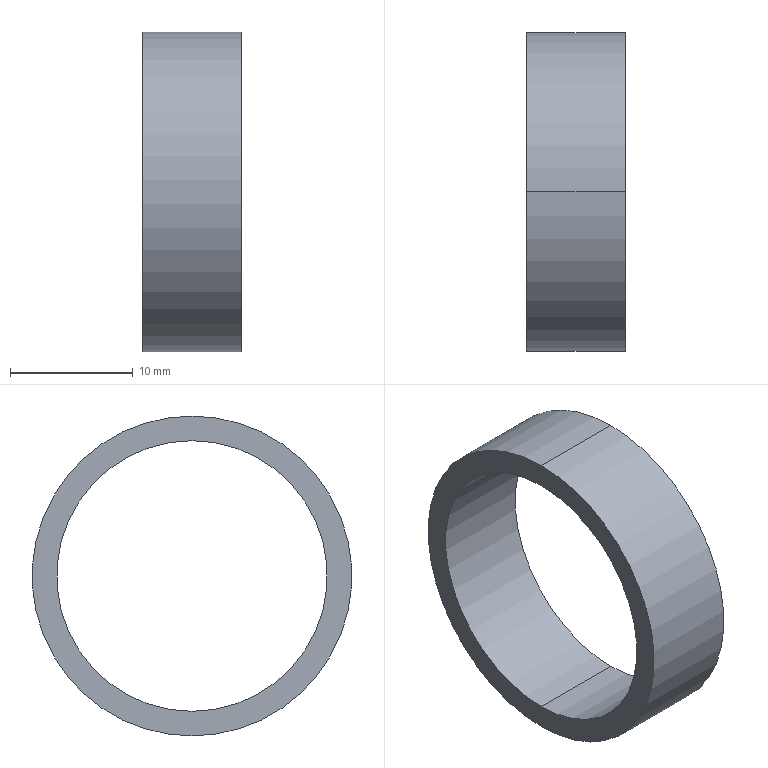Part | SolidWorks | features BaseBody 1 | 1 solid | 6 faces | box 8 x 26 x 26 mm | volume 1206 mm3 | cylinder 4 | plane 2 | commonest cylinder face diameters 22 x2 26 x2
STEP:
#1=CARTESIAN_POINT('',(-4.,0.,-13.));
#2=VERTEX_POINT('',#1);
#3=CARTESIAN_POINT('',(-4.,0.,13.));
#4=VERTEX_POINT('',#3);
#5=CARTESIAN_POINT('',(-4.,0.,0.));
#6=DIRECTION('',(1.,0.,0.));
#7=DIRECTION('',(0.,0.,-1.));
#8=AXIS2_PLACEMENT_3D('',#5,#6,#7);
#9=CIRCLE('',#8,13.);
#10=EDGE_CURVE('',#2,#4,#9,.T.);
#11=ORIENTED_EDGE('',*,*,#10,.T.);
#12=CARTESIAN_POINT('',(4.,0.,13.));
#13=VERTEX_POINT('',#12);
#14=CARTESIAN_POINT('',(-4.,0.,13.));
#15=DIRECTION('',(1.,0.,0.));
#16=VECTOR('',#15,1000.);
#17=LINE('',#14,#16);
#18=EDGE_CURVE('',#4,#13,#17,.T.);
#19=ORIENTED_EDGE('',*,*,#18,.T.);
#20=CARTESIAN_POINT('',(4.,0.,-13.));
#21=VERTEX_POINT('',#20);
#22=CARTESIAN_POINT('',(4.,0.,0.));
#23=DIRECTION('',(-1.,0.,0.));
#24=DIRECTION('',(0.,0.,-1.));
#25=AXIS2_PLACEMENT_3D('',#22,#23,#24);
#26=CIRCLE('',#25,13.);
#27=EDGE_CURVE('',#13,#21,#26,.T.);
#28=ORIENTED_EDGE('',*,*,#27,.T.);
#29=CARTESIAN_POINT('',(-4.,0.,-13.));
#30=DIRECTION('',(1.,0.,0.));
#31=VECTOR('',#30,1000.);
#32=LINE('',#29,#31);
#33=EDGE_CURVE('',#2,#21,#32,.T.);
#34=ORIENTED_EDGE('',*,*,#33,.F.);
#35=EDGE_LOOP('',(#11,#19,#28,#34));
#36=FACE_OUTER_BOUND('',#35,.T.);
#37=CARTESIAN_POINT('',(-4.,0.,0.));
#38=DIRECTION('',(1.,0.,0.));
#39=DIRECTION('',(0.,0.,-1.));
#40=AXIS2_PLACEMENT_3D('',#37,#38,#39);
#41=CYLINDRICAL_SURFACE('',#40,13.);
#42=ADVANCED_FACE('',(#36),#41,.T.);
#43=CARTESIAN_POINT('',(-4.,0.,-11.));
#44=VERTEX_POINT('',#43);
#45=CARTESIAN_POINT('',(-4.,0.,11.));
#46=VERTEX_POINT('',#45);
#47=CARTESIAN_POINT('',(-4.,0.,0.));
#48=DIRECTION('',(-1.,0.,0.));
#49=DIRECTION('',(0.,0.,-1.));
#50=AXIS2_PLACEMENT_3D('',#47,#48,#49);
#51=CIRCLE('',#50,11.);
#52=EDGE_CURVE('',#44,#46,#51,.T.);
#53=ORIENTED_EDGE('',*,*,#52,.T.);
#54=CARTESIAN_POINT('',(4.,0.,11.));
#55=VERTEX_POINT('',#54);
#56=CARTESIAN_POINT('',(-5.,0.,11.));
#57=DIRECTION('',(1.,0.,0.));
#58=VECTOR('',#57,1000.);
#59=LINE('',#56,#58);
#60=EDGE_CURVE('',#46,#55,#59,.T.);
#61=ORIENTED_EDGE('',*,*,#60,.T.);
#62=CARTESIAN_POINT('',(4.,0.,-11.));
#63=VERTEX_POINT('',#62);
#64=CARTESIAN_POINT('',(4.,0.,0.));
#65=DIRECTION('',(-1.,0.,0.));
#66=DIRECTION('',(0.,0.,-1.));
#67=AXIS2_PLACEMENT_3D('',#64,#65,#66);
#68=CIRCLE('',#67,11.);
#69=EDGE_CURVE('',#63,#55,#68,.T.);
#70=ORIENTED_EDGE('',*,*,#69,.F.);
#71=CARTESIAN_POINT('',(-5.,0.,-11.));
#72=DIRECTION('',(1.,0.,0.));
#73=VECTOR('',#72,1000.);
#74=LINE('',#71,#73);
#75=EDGE_CURVE('',#44,#63,#74,.T.);
#76=ORIENTED_EDGE('',*,*,#75,.F.);
#77=EDGE_LOOP('',(#53,#61,#70,#76));
#78=FACE_OUTER_BOUND('',#77,.T.);
#79=CARTESIAN_POINT('',(-5.,0.,0.));
#80=DIRECTION('',(1.,0.,0.));
#81=DIRECTION('',(0.,0.,-1.));
#82=AXIS2_PLACEMENT_3D('',#79,#80,#81);
#83=CYLINDRICAL_SURFACE('',#82,11.);
#84=ADVANCED_FACE('',(#78),#83,.F.);
#85=ORIENTED_EDGE('',*,*,#18,.F.);
#86=CARTESIAN_POINT('',(-4.,0.,0.));
#87=DIRECTION('',(1.,0.,0.));
#88=DIRECTION('',(0.,0.,-1.));
#89=AXIS2_PLACEMENT_3D('',#86,#87,#88);
#90=CIRCLE('',#89,13.);
#91=EDGE_CURVE('',#4,#2,#90,.T.);
#92=ORIENTED_EDGE('',*,*,#91,.T.);
#93=ORIENTED_EDGE('',*,*,#33,.T.);
#94=CARTESIAN_POINT('',(4.,0.,0.));
#95=DIRECTION('',(-1.,0.,0.));
#96=DIRECTION('',(0.,0.,-1.));
#97=AXIS2_PLACEMENT_3D('',#94,#95,#96);
#98=CIRCLE('',#97,13.);
#99=EDGE_CURVE('',#21,#13,#98,.T.);
#100=ORIENTED_EDGE('',*,*,#99,.T.);
#101=EDGE_LOOP('',(#85,#92,#93,#100));
#102=FACE_OUTER_BOUND('',#101,.T.);
#103=CARTESIAN_POINT('',(-4.,0.,0.));
#104=DIRECTION('',(1.,0.,0.));
#105=DIRECTION('',(0.,0.,-1.));
#106=AXIS2_PLACEMENT_3D('',#103,#104,#105);
#107=CYLINDRICAL_SURFACE('',#106,13.);
#108=ADVANCED_FACE('',(#102),#107,.T.);
#109=ORIENTED_EDGE('',*,*,#52,.F.);
#110=CARTESIAN_POINT('',(-4.,0.,0.));
#111=DIRECTION('',(-1.,0.,0.));
#112=DIRECTION('',(0.,0.,-1.));
#113=AXIS2_PLACEMENT_3D('',#110,#111,#112);
#114=CIRCLE('',#113,11.);
#115=EDGE_CURVE('',#46,#44,#114,.T.);
#116=ORIENTED_EDGE('',*,*,#115,.F.);
#117=EDGE_LOOP('',(#109,#116));
#118=FACE_BOUND('',#117,.T.);
#119=ORIENTED_EDGE('',*,*,#10,.F.);
#120=ORIENTED_EDGE('',*,*,#91,.F.);
#121=EDGE_LOOP('',(#119,#120));
#122=FACE_OUTER_BOUND('',#121,.T.);
#123=CARTESIAN_POINT('',(-4.,0.,0.));
#124=DIRECTION('',(1.,0.,0.));
#125=DIRECTION('',(0.,0.,-1.));
#126=AXIS2_PLACEMENT_3D('',#123,#124,#125);
#127=PLANE('',#126);
#128=ADVANCED_FACE('',(#118,#122),#127,.F.);
#129=ORIENTED_EDGE('',*,*,#69,.T.);
#130=CARTESIAN_POINT('',(4.,0.,0.));
#131=DIRECTION('',(-1.,0.,0.));
#132=DIRECTION('',(0.,0.,-1.));
#133=AXIS2_PLACEMENT_3D('',#130,#131,#132);
#134=CIRCLE('',#133,11.);
#135=EDGE_CURVE('',#55,#63,#134,.T.);
#136=ORIENTED_EDGE('',*,*,#135,.T.);
#137=EDGE_LOOP('',(#129,#136));
#138=FACE_BOUND('',#137,.T.);
#139=ORIENTED_EDGE('',*,*,#99,.F.);
#140=ORIENTED_EDGE('',*,*,#27,.F.);
#141=EDGE_LOOP('',(#139,#140));
#142=FACE_OUTER_BOUND('',#141,.T.);
#143=CARTESIAN_POINT('',(4.,0.,0.));
#144=DIRECTION('',(1.,0.,0.));
#145=DIRECTION('',(0.,0.,-1.));
#146=AXIS2_PLACEMENT_3D('',#143,#144,#145);
#147=PLANE('',#146);
#148=ADVANCED_FACE('',(#138,#142),#147,.T.);
#149=ORIENTED_EDGE('',*,*,#60,.F.);
#150=ORIENTED_EDGE('',*,*,#115,.T.);
#151=ORIENTED_EDGE('',*,*,#75,.T.);
#152=ORIENTED_EDGE('',*,*,#135,.F.);
#153=EDGE_LOOP('',(#149,#150,#151,#152));
#154=FACE_OUTER_BOUND('',#153,.T.);
#155=CARTESIAN_POINT('',(-5.,0.,0.));
#156=DIRECTION('',(1.,0.,0.));
#157=DIRECTION('',(0.,0.,-1.));
#158=AXIS2_PLACEMENT_3D('',#155,#156,#157);
#159=CYLINDRICAL_SURFACE('',#158,11.);
#160=ADVANCED_FACE('',(#154),#159,.F.);
#161=CLOSED_SHELL('',(#42,#84,#108,#128,#148,#160));
#162=MANIFOLD_SOLID_BREP('',#161);
#163=CARTESIAN_POINT('',(0.,0.,0.));
#164=DIRECTION('',(0.,0.,1.));
#165=DIRECTION('',(1.,0.,0.));
#166=AXIS2_PLACEMENT_3D('',#163,#164,#165);
#167=(LENGTH_UNIT()NAMED_UNIT(*)SI_UNIT(.MILLI.,.METRE.));
#168=UNCERTAINTY_MEASURE_WITH_UNIT(LENGTH_MEASURE(0.00001),#167,'','');
#169=(NAMED_UNIT(*)PLANE_ANGLE_UNIT()SI_UNIT($,.RADIAN.));
#170=(NAMED_UNIT(*)SI_UNIT($,.STERADIAN.)SOLID_ANGLE_UNIT());
#171=(GEOMETRIC_REPRESENTATION_CONTEXT(3)GLOBAL_UNCERTAINTY_ASSIGNED_CONTEXT((#168))GLOBAL_UNIT_ASSIGNED_CONTEXT((#167,#169,#170))REPRESENTATION_CONTEXT('',''));
#172=ADVANCED_BREP_SHAPE_REPRESENTATION('',(#162,#166),#171);